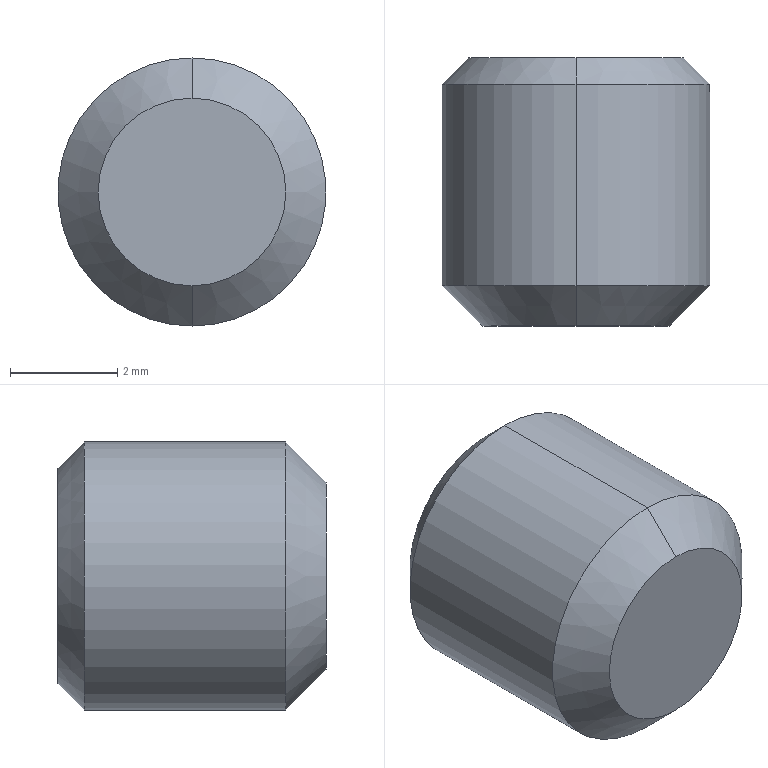Part | STEP file | 0232_Z_HOKW63_3 | 1 solid | 22 faces | box 5 x 5 x 5 mm | volume 80.427 mm3 | plane 14 | cone 6 | cylinder 2 | commonest cylinder face diameters 5 x2
STEP:
#1=CARTESIAN_POINT('',(0.,0.,0.));
#2=DIRECTION('',(0.,0.,1.));
#3=DIRECTION('',(1.,0.,0.));
#4=AXIS2_PLACEMENT_3D('',#1,#2,#3);
#5=CARTESIAN_POINT('',(-9.,17.009,-2.5));
#6=VERTEX_POINT('',#5);
#7=CARTESIAN_POINT('',(-9.,17.009,2.5));
#8=VERTEX_POINT('',#7);
#9=CARTESIAN_POINT('',(-9.,17.009,0.));
#10=DIRECTION('',(0.,-1.,0.));
#11=DIRECTION('',(0.,0.,-1.));
#12=AXIS2_PLACEMENT_3D('',#9,#10,#11);
#13=CIRCLE('',#12,2.5);
#14=CARTESIAN_POINT('',(-9.,15.13,0.));
#15=DIRECTION('',(0.,-1.,0.));
#16=DIRECTION('',(0.,0.,-1.));
#17=AXIS2_PLACEMENT_3D('',#14,#15,#16);
#18=CYLINDRICAL_SURFACE('',#17,2.5);
#19=CARTESIAN_POINT('',(0.,-1.88));
#20=DIRECTION('',(1.,0.));
#21=VECTOR('',#20,1.);
#22=LINE('',#19,#21);
#23=(GEOMETRIC_REPRESENTATION_CONTEXT(2)PARAMETRIC_REPRESENTATION_CONTEXT()REPRESENTATION_CONTEXT('',''));
#24=DEFINITIONAL_REPRESENTATION('',(#22),#23);
#25=PCURVE('',#18,#24);
#26=CARTESIAN_POINT('',(-9.,17.01,0.));
#27=DIRECTION('',(0.,-1.,0.));
#28=DIRECTION('',(0.,0.,-1.));
#29=AXIS2_PLACEMENT_3D('',#26,#27,#28);
#30=CONICAL_SURFACE('',#29,2.5,0.7854);
#31=CARTESIAN_POINT('',(0.,0.));
#32=DIRECTION('',(1.,0.));
#33=VECTOR('',#32,1.);
#34=LINE('',#31,#33);
#35=(GEOMETRIC_REPRESENTATION_CONTEXT(2)PARAMETRIC_REPRESENTATION_CONTEXT()REPRESENTATION_CONTEXT('',''));
#36=DEFINITIONAL_REPRESENTATION('',(#34),#35);
#37=PCURVE('',#30,#36);
#38=SURFACE_CURVE('',#13,(#25,#37),.PCURVE_S1.);
#39=EDGE_CURVE('',#6,#8,#38,.T.);
#40=ORIENTED_EDGE('',*,*,#39,.T.);
#41=CARTESIAN_POINT('',(-9.,13.25,2.5));
#42=VERTEX_POINT('',#41);
#43=CARTESIAN_POINT('',(-9.,15.13,2.5));
#44=DIRECTION('',(0.,-1.,0.));
#45=VECTOR('',#44,1.);
#46=LINE('',#43,#45);
#47=CARTESIAN_POINT('',(3.142,0.));
#48=DIRECTION('',(0.,1.));
#49=VECTOR('',#48,1.);
#50=LINE('',#47,#49);
#51=(GEOMETRIC_REPRESENTATION_CONTEXT(2)PARAMETRIC_REPRESENTATION_CONTEXT()REPRESENTATION_CONTEXT('',''));
#52=DEFINITIONAL_REPRESENTATION('',(#50),#51);
#53=PCURVE('',#18,#52);
#54=CARTESIAN_POINT('',(-9.,15.13,0.));
#55=DIRECTION('',(0.,-1.,0.));
#56=DIRECTION('',(0.,0.,-1.));
#57=AXIS2_PLACEMENT_3D('',#54,#55,#56);
#58=CYLINDRICAL_SURFACE('',#57,2.5);
#59=CARTESIAN_POINT('',(3.142,0.));
#60=DIRECTION('',(0.,1.));
#61=VECTOR('',#60,1.);
#62=LINE('',#59,#61);
#63=(GEOMETRIC_REPRESENTATION_CONTEXT(2)PARAMETRIC_REPRESENTATION_CONTEXT()REPRESENTATION_CONTEXT('',''));
#64=DEFINITIONAL_REPRESENTATION('',(#62),#63);
#65=PCURVE('',#58,#64);
#66=SURFACE_CURVE('',#46,(#53,#65),.PCURVE_S1.);
#67=EDGE_CURVE('',#8,#42,#66,.T.);
#68=ORIENTED_EDGE('',*,*,#67,.T.);
#69=CARTESIAN_POINT('',(-9.,13.25,-2.5));
#70=VERTEX_POINT('',#69);
#71=CARTESIAN_POINT('',(-9.,13.25,0.));
#72=DIRECTION('',(0.,1.,0.));
#73=DIRECTION('',(0.,0.,-1.));
#74=AXIS2_PLACEMENT_3D('',#71,#72,#73);
#75=CIRCLE('',#74,2.5);
#76=CARTESIAN_POINT('',(6.283,1.88));
#77=DIRECTION('',(-1.,0.));
#78=VECTOR('',#77,1.);
#79=LINE('',#76,#78);
#80=(GEOMETRIC_REPRESENTATION_CONTEXT(2)PARAMETRIC_REPRESENTATION_CONTEXT()REPRESENTATION_CONTEXT('',''));
#81=DEFINITIONAL_REPRESENTATION('',(#79),#80);
#82=PCURVE('',#18,#81);
#83=CARTESIAN_POINT('',(-9.,13.25,0.));
#84=DIRECTION('',(0.,1.,0.));
#85=DIRECTION('',(0.,0.,1.));
#86=AXIS2_PLACEMENT_3D('',#83,#84,#85);
#87=CONICAL_SURFACE('',#86,2.5,0.7854);
#88=CARTESIAN_POINT('',(-3.142,0.));
#89=DIRECTION('',(1.,0.));
#90=VECTOR('',#89,1.);
#91=LINE('',#88,#90);
#92=(GEOMETRIC_REPRESENTATION_CONTEXT(2)PARAMETRIC_REPRESENTATION_CONTEXT()REPRESENTATION_CONTEXT('',''));
#93=DEFINITIONAL_REPRESENTATION('',(#91),#92);
#94=PCURVE('',#87,#93);
#95=SURFACE_CURVE('',#75,(#82,#94),.PCURVE_S1.);
#96=EDGE_CURVE('',#42,#70,#95,.T.);
#97=ORIENTED_EDGE('',*,*,#96,.T.);
#98=CARTESIAN_POINT('',(-9.,15.13,-2.5));
#99=DIRECTION('',(0.,-1.,0.));
#100=VECTOR('',#99,1.);
#101=LINE('',#98,#100);
#102=CARTESIAN_POINT('',(0.,0.));
#103=DIRECTION('',(0.,1.));
#104=VECTOR('',#103,1.);
#105=LINE('',#102,#104);
#106=(GEOMETRIC_REPRESENTATION_CONTEXT(2)PARAMETRIC_REPRESENTATION_CONTEXT()REPRESENTATION_CONTEXT('',''));
#107=DEFINITIONAL_REPRESENTATION('',(#105),#106);
#108=PCURVE('',#18,#107);
#109=CARTESIAN_POINT('',(6.283,0.));
#110=DIRECTION('',(0.,1.));
#111=VECTOR('',#110,1.);
#112=LINE('',#109,#111);
#113=(GEOMETRIC_REPRESENTATION_CONTEXT(2)PARAMETRIC_REPRESENTATION_CONTEXT()REPRESENTATION_CONTEXT('',''));
#114=DEFINITIONAL_REPRESENTATION('',(#112),#113);
#115=PCURVE('',#58,#114);
#116=SURFACE_CURVE('',#101,(#108,#115),.PCURVE_S1.);
#117=EDGE_CURVE('',#6,#70,#116,.T.);
#118=ORIENTED_EDGE('',*,*,#117,.F.);
#119=EDGE_LOOP('',(#40,#68,#97,#118));
#120=FACE_BOUND('',#119,.T.);
#121=ADVANCED_FACE('',(#120),#18,.T.);
#122=CARTESIAN_POINT('',(-9.,17.5,-2.009));
#123=VERTEX_POINT('',#122);
#124=CARTESIAN_POINT('',(-9.,17.5,2.009));
#125=VERTEX_POINT('',#124);
#126=CARTESIAN_POINT('',(-9.,17.5,0.));
#127=DIRECTION('',(0.,-1.,0.));
#128=DIRECTION('',(0.,0.,-1.));
#129=AXIS2_PLACEMENT_3D('',#126,#127,#128);
#130=CIRCLE('',#129,2.009);
#131=CARTESIAN_POINT('',(0.,-0.4905));
#132=DIRECTION('',(1.,0.));
#133=VECTOR('',#132,1.);
#134=LINE('',#131,#133);
#135=(GEOMETRIC_REPRESENTATION_CONTEXT(2)PARAMETRIC_REPRESENTATION_CONTEXT()REPRESENTATION_CONTEXT('',''));
#136=DEFINITIONAL_REPRESENTATION('',(#134),#135);
#137=PCURVE('',#30,#136);
#138=CARTESIAN_POINT('',(-9.,17.5,1.005));
#139=DIRECTION('',(0.,1.,0.));
#140=DIRECTION('',(0.,0.,1.));
#141=AXIS2_PLACEMENT_3D('',#138,#139,#140);
#142=PLANE('',#141);
#143=CARTESIAN_POINT('',(-3.014,0.));
#144=CARTESIAN_POINT('',(-3.014,3.481));
#145=CARTESIAN_POINT('',(0.,1.74));
#146=CARTESIAN_POINT('',(3.014,0.));
#147=CARTESIAN_POINT('',(0.,-1.74));
#148=CARTESIAN_POINT('',(-3.014,-3.481));
#149=CARTESIAN_POINT('',(-3.014,0.));
#150=(BOUNDED_CURVE()B_SPLINE_CURVE(2,(#143,#144,#145,#146,#147,#148,#149),.UNSPECIFIED.,.T.,.F.)B_SPLINE_CURVE_WITH_KNOTS((1,2,2,2,2,1),(-2.094,0.,2.094,4.189,6.283,8.378),.UNSPECIFIED.)CURVE()GEOMETRIC_REPRESENTATION_ITEM()RATIONAL_B_SPLINE_CURVE((1.,0.5,1.,0.5,1.,0.5,1.))REPRESENTATION_ITEM(''));
#151=(GEOMETRIC_REPRESENTATION_CONTEXT(2)PARAMETRIC_REPRESENTATION_CONTEXT()REPRESENTATION_CONTEXT('',''));
#152=DEFINITIONAL_REPRESENTATION('',(#150),#151);
#153=PCURVE('',#142,#152);
#154=SURFACE_CURVE('',#130,(#137,#153),.PCURVE_S1.);
#155=EDGE_CURVE('',#123,#125,#154,.T.);
#156=ORIENTED_EDGE('',*,*,#155,.T.);
#157=CARTESIAN_POINT('',(-9.,17.01,2.5));
#158=DIRECTION('',(0.,-0.7071,0.7071));
#159=VECTOR('',#158,1.);
#160=LINE('',#157,#159);
#161=CARTESIAN_POINT('',(3.142,0.));
#162=DIRECTION('',(0.,1.));
#163=VECTOR('',#162,1.);
#164=LINE('',#161,#163);
#165=(GEOMETRIC_REPRESENTATION_CONTEXT(2)PARAMETRIC_REPRESENTATION_CONTEXT()REPRESENTATION_CONTEXT('',''));
#166=DEFINITIONAL_REPRESENTATION('',(#164),#165);
#167=PCURVE('',#30,#166);
#168=CARTESIAN_POINT('',(-9.,17.01,0.));
#169=DIRECTION('',(0.,-1.,0.));
#170=DIRECTION('',(0.,0.,-1.));
#171=AXIS2_PLACEMENT_3D('',#168,#169,#170);
#172=CONICAL_SURFACE('',#171,2.5,0.7854);
#173=CARTESIAN_POINT('',(3.142,0.));
#174=DIRECTION('',(0.,1.));
#175=VECTOR('',#174,1.);
#176=LINE('',#173,#175);
#177=(GEOMETRIC_REPRESENTATION_CONTEXT(2)PARAMETRIC_REPRESENTATION_CONTEXT()REPRESENTATION_CONTEXT('',''));
#178=DEFINITIONAL_REPRESENTATION('',(#176),#177);
#179=PCURVE('',#172,#178);
#180=SURFACE_CURVE('',#160,(#167,#179),.PCURVE_S1.);
#181=EDGE_CURVE('',#125,#8,#180,.T.);
#182=ORIENTED_EDGE('',*,*,#181,.T.);
#183=ORIENTED_EDGE('',*,*,#39,.F.);
#184=CARTESIAN_POINT('',(-9.,17.01,-2.5));
#185=DIRECTION('',(0.,-0.7071,-0.7071));
#186=VECTOR('',#185,1.);
#187=LINE('',#184,#186);
#188=CARTESIAN_POINT('',(0.,0.));
#189=DIRECTION('',(0.,1.));
#190=VECTOR('',#189,1.);
#191=LINE('',#188,#190);
#192=(GEOMETRIC_REPRESENTATION_CONTEXT(2)PARAMETRIC_REPRESENTATION_CONTEXT()REPRESENTATION_CONTEXT('',''));
#193=DEFINITIONAL_REPRESENTATION('',(#191),#192);
#194=PCURVE('',#30,#193);
#195=CARTESIAN_POINT('',(6.283,0.));
#196=DIRECTION('',(0.,1.));
#197=VECTOR('',#196,1.);
#198=LINE('',#195,#197);
#199=(GEOMETRIC_REPRESENTATION_CONTEXT(2)PARAMETRIC_REPRESENTATION_CONTEXT()REPRESENTATION_CONTEXT('',''));
#200=DEFINITIONAL_REPRESENTATION('',(#198),#199);
#201=PCURVE('',#172,#200);
#202=SURFACE_CURVE('',#187,(#194,#201),.PCURVE_S1.);
#203=EDGE_CURVE('',#123,#6,#202,.T.);
#204=ORIENTED_EDGE('',*,*,#203,.F.);
#205=EDGE_LOOP('',(#156,#182,#183,#204));
#206=FACE_BOUND('',#205,.T.);
#207=ADVANCED_FACE('',(#206),#30,.T.);
#208=CARTESIAN_POINT('',(-9.,12.5,1.75));
#209=VERTEX_POINT('',#208);
#210=CARTESIAN_POINT('',(-9.,12.5,-1.75));
#211=VERTEX_POINT('',#210);
#212=CARTESIAN_POINT('',(-9.,12.5,0.));
#213=DIRECTION('',(0.,1.,0.));
#214=DIRECTION('',(0.,0.,1.));
#215=AXIS2_PLACEMENT_3D('',#212,#213,#214);
#216=CIRCLE('',#215,1.75);
#217=CARTESIAN_POINT('',(0.,-0.75));
#218=DIRECTION('',(1.,0.));
#219=VECTOR('',#218,1.);
#220=LINE('',#217,#219);
#221=(GEOMETRIC_REPRESENTATION_CONTEXT(2)PARAMETRIC_REPRESENTATION_CONTEXT()REPRESENTATION_CONTEXT('',''));
#222=DEFINITIONAL_REPRESENTATION('',(#220),#221);
#223=PCURVE('',#87,#222);
#224=CARTESIAN_POINT('',(-9.,12.5,0.875));
#225=DIRECTION('',(0.,-1.,0.));
#226=DIRECTION('',(0.,0.,-1.));
#227=AXIS2_PLACEMENT_3D('',#224,#225,#226);
#228=PLANE('',#227);
#229=CARTESIAN_POINT('',(-0.875,0.));
#230=CARTESIAN_POINT('',(-0.875,3.031));
#231=CARTESIAN_POINT('',(1.75,1.516));
#232=CARTESIAN_POINT('',(4.375,0.));
#233=CARTESIAN_POINT('',(1.75,-1.516));
#234=CARTESIAN_POINT('',(-0.875,-3.031));
#235=CARTESIAN_POINT('',(-0.875,0.));
#236=(BOUNDED_CURVE()B_SPLINE_CURVE(2,(#229,#230,#231,#232,#233,#234,#235),.UNSPECIFIED.,.T.,.F.)B_SPLINE_CURVE_WITH_KNOTS((1,2,2,2,2,1),(-2.094,0.,2.094,4.189,6.283,8.378),.UNSPECIFIED.)CURVE()GEOMETRIC_REPRESENTATION_ITEM()RATIONAL_B_SPLINE_CURVE((1.,0.5,1.,0.5,1.,0.5,1.))REPRESENTATION_ITEM(''));
#237=(GEOMETRIC_REPRESENTATION_CONTEXT(2)PARAMETRIC_REPRESENTATION_CONTEXT()REPRESENTATION_CONTEXT('',''));
#238=DEFINITIONAL_REPRESENTATION('',(#236),#237);
#239=PCURVE('',#228,#238);
#240=SURFACE_CURVE('',#216,(#223,#239),.PCURVE_S1.);
#241=EDGE_CURVE('',#209,#211,#240,.T.);
#242=ORIENTED_EDGE('',*,*,#241,.T.);
#243=CARTESIAN_POINT('',(-9.,13.25,-2.5));
#244=DIRECTION('',(0.,0.7071,-0.7071));
#245=VECTOR('',#244,1.);
#246=LINE('',#243,#245);
#247=CARTESIAN_POINT('',(3.142,0.));
#248=DIRECTION('',(0.,1.));
#249=VECTOR('',#248,1.);
#250=LINE('',#247,#249);
#251=(GEOMETRIC_REPRESENTATION_CONTEXT(2)PARAMETRIC_REPRESENTATION_CONTEXT()REPRESENTATION_CONTEXT('',''));
#252=DEFINITIONAL_REPRESENTATION('',(#250),#251);
#253=PCURVE('',#87,#252);
#254=CARTESIAN_POINT('',(-9.,13.25,0.));
#255=DIRECTION('',(0.,1.,0.));
#256=DIRECTION('',(0.,0.,1.));
#257=AXIS2_PLACEMENT_3D('',#254,#255,#256);
#258=CONICAL_SURFACE('',#257,2.5,0.7854);
#259=CARTESIAN_POINT('',(3.142,0.));
#260=DIRECTION('',(0.,1.));
#261=VECTOR('',#260,1.);
#262=LINE('',#259,#261);
#263=(GEOMETRIC_REPRESENTATION_CONTEXT(2)PARAMETRIC_REPRESENTATION_CONTEXT()REPRESENTATION_CONTEXT('',''));
#264=DEFINITIONAL_REPRESENTATION('',(#262),#263);
#265=PCURVE('',#258,#264);
#266=SURFACE_CURVE('',#246,(#253,#265),.PCURVE_S1.);
#267=EDGE_CURVE('',#211,#70,#266,.T.);
#268=ORIENTED_EDGE('',*,*,#267,.T.);
#269=ORIENTED_EDGE('',*,*,#96,.F.);
#270=CARTESIAN_POINT('',(-9.,13.25,2.5));
#271=DIRECTION('',(0.,0.7071,0.7071));
#272=VECTOR('',#271,1.);
#273=LINE('',#270,#272);
#274=CARTESIAN_POINT('',(0.,0.));
#275=DIRECTION('',(0.,1.));
#276=VECTOR('',#275,1.);
#277=LINE('',#274,#276);
#278=(GEOMETRIC_REPRESENTATION_CONTEXT(2)PARAMETRIC_REPRESENTATION_CONTEXT()REPRESENTATION_CONTEXT('',''));
#279=DEFINITIONAL_REPRESENTATION('',(#277),#278);
#280=PCURVE('',#87,#279);
#281=CARTESIAN_POINT('',(6.283,0.));
#282=DIRECTION('',(0.,1.));
#283=VECTOR('',#282,1.);
#284=LINE('',#281,#283);
#285=(GEOMETRIC_REPRESENTATION_CONTEXT(2)PARAMETRIC_REPRESENTATION_CONTEXT()REPRESENTATION_CONTEXT('',''));
#286=DEFINITIONAL_REPRESENTATION('',(#284),#285);
#287=PCURVE('',#258,#286);
#288=SURFACE_CURVE('',#273,(#280,#287),.PCURVE_S1.);
#289=EDGE_CURVE('',#209,#42,#288,.T.);
#290=ORIENTED_EDGE('',*,*,#289,.F.);
#291=EDGE_LOOP('',(#242,#268,#269,#290));
#292=FACE_BOUND('',#291,.T.);
#293=ADVANCED_FACE('',(#292),#87,.T.);
#294=CARTESIAN_POINT('',(-9.,15.5,1.25));
#295=VERTEX_POINT('',#294);
#296=CARTESIAN_POINT('',(-9.625,15.5,1.083));
#297=VERTEX_POINT('',#296);
#298=CARTESIAN_POINT('',(-9.,15.5,0.));
#299=DIRECTION('',(0.,-1.,0.));
#300=DIRECTION('',(0.,0.,1.));
#301=AXIS2_PLACEMENT_3D('',#298,#299,#300);
#302=CIRCLE('',#301,1.25);
#303=CARTESIAN_POINT('',(-9.,15.5,0.));
#304=DIRECTION('',(0.,1.,0.));
#305=DIRECTION('',(0.,0.,1.));
#306=AXIS2_PLACEMENT_3D('',#303,#304,#305);
#307=CONICAL_SURFACE('',#306,1.25,1.047);
#308=CARTESIAN_POINT('',(6.283,0.));
#309=DIRECTION('',(-1.,0.));
#310=VECTOR('',#309,1.);
#311=LINE('',#308,#310);
#312=(GEOMETRIC_REPRESENTATION_CONTEXT(2)PARAMETRIC_REPRESENTATION_CONTEXT()REPRESENTATION_CONTEXT('',''));
#313=DEFINITIONAL_REPRESENTATION('',(#311),#312);
#314=PCURVE('',#307,#313);
#315=CARTESIAN_POINT('',(-9.,15.5,0.));
#316=DIRECTION('',(0.,-1.,0.));
#317=DIRECTION('',(0.,0.,-1.));
#318=AXIS2_PLACEMENT_3D('',#315,#316,#317);
#319=PLANE('',#318);
#320=CARTESIAN_POINT('',(0.,0.));
#321=DIRECTION('',(-1.,0.));
#322=AXIS2_PLACEMENT_2D('',#320,#321);
#323=CIRCLE('',#322,1.25);
#324=(GEOMETRIC_REPRESENTATION_CONTEXT(2)PARAMETRIC_REPRESENTATION_CONTEXT()REPRESENTATION_CONTEXT('',''));
#325=DEFINITIONAL_REPRESENTATION('',(#323),#324);
#326=PCURVE('',#319,#325);
#327=SURFACE_CURVE('',#302,(#314,#326),.PCURVE_S1.);
#328=EDGE_CURVE('',#295,#297,#327,.T.);
#329=ORIENTED_EDGE('',*,*,#328,.T.);
#330=CARTESIAN_POINT('',(-10.25,15.5,0.));
#331=VERTEX_POINT('',#330);
#332=CARTESIAN_POINT('',(-9.,15.5,0.));
#333=DIRECTION('',(0.,1.,0.));
#334=DIRECTION('',(0.,0.,1.));
#335=AXIS2_PLACEMENT_3D('',#332,#333,#334);
#336=CIRCLE('',#335,1.25);
#337=CARTESIAN_POINT('',(0.,0.));
#338=DIRECTION('',(1.,0.));
#339=VECTOR('',#338,1.);
#340=LINE('',#337,#339);
#341=(GEOMETRIC_REPRESENTATION_CONTEXT(2)PARAMETRIC_REPRESENTATION_CONTEXT()REPRESENTATION_CONTEXT('',''));
#342=DEFINITIONAL_REPRESENTATION('',(#340),#341);
#343=PCURVE('',#307,#342);
#344=CARTESIAN_POINT('',(-9.,15.5,0.));
#345=DIRECTION('',(0.,-1.,0.));
#346=DIRECTION('',(0.,0.,-1.));
#347=AXIS2_PLACEMENT_3D('',#344,#345,#346);
#348=PLANE('',#347);
#349=CARTESIAN_POINT('',(-1.25,0.));
#350=CARTESIAN_POINT('',(-1.25,2.165));
#351=CARTESIAN_POINT('',(0.625,1.083));
#352=CARTESIAN_POINT('',(2.5,0.));
#353=CARTESIAN_POINT('',(0.625,-1.083));
#354=CARTESIAN_POINT('',(-1.25,-2.165));
#355=CARTESIAN_POINT('',(-1.25,0.));
#356=(BOUNDED_CURVE()B_SPLINE_CURVE(2,(#349,#350,#351,#352,#353,#354,#355),.UNSPECIFIED.,.T.,.F.)B_SPLINE_CURVE_WITH_KNOTS((1,2,2,2,2,1),(-2.094,0.,2.094,4.189,6.283,8.378),.UNSPECIFIED.)CURVE()GEOMETRIC_REPRESENTATION_ITEM()RATIONAL_B_SPLINE_CURVE((1.,0.5,1.,0.5,1.,0.5,1.))REPRESENTATION_ITEM(''));
#357=(GEOMETRIC_REPRESENTATION_CONTEXT(2)PARAMETRIC_REPRESENTATION_CONTEXT()REPRESENTATION_CONTEXT('',''));
#358=DEFINITIONAL_REPRESENTATION('',(#356),#357);
#359=PCURVE('',#348,#358);
#360=SURFACE_CURVE('',#336,(#343,#359),.PCURVE_S1.);
#361=EDGE_CURVE('',#331,#297,#360,.T.);
#362=ORIENTED_EDGE('',*,*,#361,.F.);
#363=CARTESIAN_POINT('',(-9.625,15.5,-1.083));
#364=VERTEX_POINT('',#363);
#365=CARTESIAN_POINT('',(-9.,15.5,0.));
#366=DIRECTION('',(0.,-1.,0.));
#367=DIRECTION('',(0.,0.,1.));
#368=AXIS2_PLACEMENT_3D('',#365,#366,#367);
#369=CIRCLE('',#368,1.25);
#370=CARTESIAN_POINT('',(6.283,0.));
#371=DIRECTION('',(-1.,0.));
#372=VECTOR('',#371,1.);
#373=LINE('',#370,#372);
#374=(GEOMETRIC_REPRESENTATION_CONTEXT(2)PARAMETRIC_REPRESENTATION_CONTEXT()REPRESENTATION_CONTEXT('',''));
#375=DEFINITIONAL_REPRESENTATION('',(#373),#374);
#376=PCURVE('',#307,#375);
#377=CARTESIAN_POINT('',(-9.,15.5,0.));
#378=DIRECTION('',(0.,-1.,0.));
#379=DIRECTION('',(0.,0.,-1.));
#380=AXIS2_PLACEMENT_3D('',#377,#378,#379);
#381=PLANE('',#380);
#382=CARTESIAN_POINT('',(0.,0.));
#383=DIRECTION('',(-1.,0.));
#384=AXIS2_PLACEMENT_2D('',#382,#383);
#385=CIRCLE('',#384,1.25);
#386=(GEOMETRIC_REPRESENTATION_CONTEXT(2)PARAMETRIC_REPRESENTATION_CONTEXT()REPRESENTATION_CONTEXT('',''));
#387=DEFINITIONAL_REPRESENTATION('',(#385),#386);
#388=PCURVE('',#381,#387);
#389=SURFACE_CURVE('',#369,(#376,#388),.PCURVE_S1.);
#390=EDGE_CURVE('',#331,#364,#389,.T.);
#391=ORIENTED_EDGE('',*,*,#390,.T.);
#392=CARTESIAN_POINT('',(-9.,15.5,-1.25));
#393=VERTEX_POINT('',#392);
#394=CARTESIAN_POINT('',(-9.,15.5,0.));
#395=DIRECTION('',(0.,-1.,0.));
#396=DIRECTION('',(0.,0.,1.));
#397=AXIS2_PLACEMENT_3D('',#394,#395,#396);
#398=CIRCLE('',#397,1.25);
#399=CARTESIAN_POINT('',(6.283,0.));
#400=DIRECTION('',(-1.,0.));
#401=VECTOR('',#400,1.);
#402=LINE('',#399,#401);
#403=(GEOMETRIC_REPRESENTATION_CONTEXT(2)PARAMETRIC_REPRESENTATION_CONTEXT()REPRESENTATION_CONTEXT('',''));
#404=DEFINITIONAL_REPRESENTATION('',(#402),#403);
#405=PCURVE('',#307,#404);
#406=CARTESIAN_POINT('',(-9.,15.5,0.));
#407=DIRECTION('',(0.,-1.,0.));
#408=DIRECTION('',(0.,0.,-1.));
#409=AXIS2_PLACEMENT_3D('',#406,#407,#408);
#410=PLANE('',#409);
#411=CARTESIAN_POINT('',(0.,0.));
#412=DIRECTION('',(-1.,0.));
#413=AXIS2_PLACEMENT_2D('',#411,#412);
#414=CIRCLE('',#413,1.25);
#415=(GEOMETRIC_REPRESENTATION_CONTEXT(2)PARAMETRIC_REPRESENTATION_CONTEXT()REPRESENTATION_CONTEXT('',''));
#416=DEFINITIONAL_REPRESENTATION('',(#414),#415);
#417=PCURVE('',#410,#416);
#418=SURFACE_CURVE('',#398,(#405,#417),.PCURVE_S1.);
#419=EDGE_CURVE('',#364,#393,#418,.T.);
#420=ORIENTED_EDGE('',*,*,#419,.T.);
#421=CARTESIAN_POINT('',(-9.,14.778,0.));
#422=VERTEX_POINT('',#421);
#423=CARTESIAN_POINT('',(-9.,15.5,-1.25));
#424=DIRECTION('',(0.,0.5,-0.866));
#425=VECTOR('',#424,1.);
#426=LINE('',#423,#425);
#427=CARTESIAN_POINT('',(3.142,0.));
#428=DIRECTION('',(0.,1.));
#429=VECTOR('',#428,1.);
#430=LINE('',#427,#429);
#431=(GEOMETRIC_REPRESENTATION_CONTEXT(2)PARAMETRIC_REPRESENTATION_CONTEXT()REPRESENTATION_CONTEXT('',''));
#432=DEFINITIONAL_REPRESENTATION('',(#430),#431);
#433=PCURVE('',#307,#432);
#434=CARTESIAN_POINT('',(-9.,15.5,0.));
#435=DIRECTION('',(0.,1.,0.));
#436=DIRECTION('',(0.,0.,1.));
#437=AXIS2_PLACEMENT_3D('',#434,#435,#436);
#438=CONICAL_SURFACE('',#437,1.25,1.047);
#439=CARTESIAN_POINT('',(3.142,0.));
#440=DIRECTION('',(0.,1.));
#441=VECTOR('',#440,1.);
#442=LINE('',#439,#441);
#443=(GEOMETRIC_REPRESENTATION_CONTEXT(2)PARAMETRIC_REPRESENTATION_CONTEXT()REPRESENTATION_CONTEXT('',''));
#444=DEFINITIONAL_REPRESENTATION('',(#442),#443);
#445=PCURVE('',#438,#444);
#446=SURFACE_CURVE('',#426,(#433,#445),.PCURVE_S1.);
#447=EDGE_CURVE('',#422,#393,#446,.T.);
#448=ORIENTED_EDGE('',*,*,#447,.F.);
#449=CARTESIAN_POINT('',(-9.,15.5,1.25));
#450=DIRECTION('',(0.,0.5,0.866));
#451=VECTOR('',#450,1.);
#452=LINE('',#449,#451);
#453=CARTESIAN_POINT('',(6.283,0.));
#454=DIRECTION('',(0.,1.));
#455=VECTOR('',#454,1.);
#456=LINE('',#453,#455);
#457=(GEOMETRIC_REPRESENTATION_CONTEXT(2)PARAMETRIC_REPRESENTATION_CONTEXT()REPRESENTATION_CONTEXT('',''));
#458=DEFINITIONAL_REPRESENTATION('',(#456),#457);
#459=PCURVE('',#307,#458);
#460=CARTESIAN_POINT('',(0.,0.));
#461=DIRECTION('',(0.,1.));
#462=VECTOR('',#461,1.);
#463=LINE('',#460,#462);
#464=(GEOMETRIC_REPRESENTATION_CONTEXT(2)PARAMETRIC_REPRESENTATION_CONTEXT()REPRESENTATION_CONTEXT('',''));
#465=DEFINITIONAL_REPRESENTATION('',(#463),#464);
#466=PCURVE('',#438,#465);
#467=SURFACE_CURVE('',#452,(#459,#466),.PCURVE_S1.);
#468=EDGE_CURVE('',#422,#295,#467,.T.);
#469=ORIENTED_EDGE('',*,*,#468,.T.);
#470=EDGE_LOOP('',(#329,#362,#391,#420,#448,#469));
#471=FACE_BOUND('',#470,.F.);
#472=ADVANCED_FACE('',(#471),#307,.F.);
#473=ORIENTED_EDGE('',*,*,#67,.F.);
#474=CARTESIAN_POINT('',(-9.,17.009,0.));
#475=DIRECTION('',(0.,-1.,0.));
#476=DIRECTION('',(0.,0.,-1.));
#477=AXIS2_PLACEMENT_3D('',#474,#475,#476);
#478=CIRCLE('',#477,2.5);
#479=CARTESIAN_POINT('',(0.,-1.88));
#480=DIRECTION('',(1.,0.));
#481=VECTOR('',#480,1.);
#482=LINE('',#479,#481);
#483=(GEOMETRIC_REPRESENTATION_CONTEXT(2)PARAMETRIC_REPRESENTATION_CONTEXT()REPRESENTATION_CONTEXT('',''));
#484=DEFINITIONAL_REPRESENTATION('',(#482),#483);
#485=PCURVE('',#58,#484);
#486=CARTESIAN_POINT('',(0.,0.));
#487=DIRECTION('',(1.,0.));
#488=VECTOR('',#487,1.);
#489=LINE('',#486,#488);
#490=(GEOMETRIC_REPRESENTATION_CONTEXT(2)PARAMETRIC_REPRESENTATION_CONTEXT()REPRESENTATION_CONTEXT('',''));
#491=DEFINITIONAL_REPRESENTATION('',(#489),#490);
#492=PCURVE('',#172,#491);
#493=SURFACE_CURVE('',#478,(#485,#492),.PCURVE_S1.);
#494=EDGE_CURVE('',#8,#6,#493,.T.);
#495=ORIENTED_EDGE('',*,*,#494,.T.);
#496=ORIENTED_EDGE('',*,*,#117,.T.);
#497=CARTESIAN_POINT('',(-9.,13.25,0.));
#498=DIRECTION('',(0.,1.,0.));
#499=DIRECTION('',(0.,0.,-1.));
#500=AXIS2_PLACEMENT_3D('',#497,#498,#499);
#501=CIRCLE('',#500,2.5);
#502=CARTESIAN_POINT('',(6.283,1.88));
#503=DIRECTION('',(-1.,0.));
#504=VECTOR('',#503,1.);
#505=LINE('',#502,#504);
#506=(GEOMETRIC_REPRESENTATION_CONTEXT(2)PARAMETRIC_REPRESENTATION_CONTEXT()REPRESENTATION_CONTEXT('',''));
#507=DEFINITIONAL_REPRESENTATION('',(#505),#506);
#508=PCURVE('',#58,#507);
#509=CARTESIAN_POINT('',(3.142,0.));
#510=DIRECTION('',(1.,0.));
#511=VECTOR('',#510,1.);
#512=LINE('',#509,#511);
#513=(GEOMETRIC_REPRESENTATION_CONTEXT(2)PARAMETRIC_REPRESENTATION_CONTEXT()REPRESENTATION_CONTEXT('',''));
#514=DEFINITIONAL_REPRESENTATION('',(#512),#513);
#515=PCURVE('',#258,#514);
#516=SURFACE_CURVE('',#501,(#508,#515),.PCURVE_S1.);
#517=EDGE_CURVE('',#70,#42,#516,.T.);
#518=ORIENTED_EDGE('',*,*,#517,.T.);
#519=EDGE_LOOP('',(#473,#495,#496,#518));
#520=FACE_BOUND('',#519,.T.);
#521=ADVANCED_FACE('',(#520),#58,.T.);
#522=ORIENTED_EDGE('',*,*,#181,.F.);
#523=CARTESIAN_POINT('',(-9.,17.5,0.));
#524=DIRECTION('',(0.,-1.,0.));
#525=DIRECTION('',(0.,0.,-1.));
#526=AXIS2_PLACEMENT_3D('',#523,#524,#525);
#527=CIRCLE('',#526,2.009);
#528=CARTESIAN_POINT('',(0.,-0.4905));
#529=DIRECTION('',(1.,0.));
#530=VECTOR('',#529,1.);
#531=LINE('',#528,#530);
#532=(GEOMETRIC_REPRESENTATION_CONTEXT(2)PARAMETRIC_REPRESENTATION_CONTEXT()REPRESENTATION_CONTEXT('',''));
#533=DEFINITIONAL_REPRESENTATION('',(#531),#532);
#534=PCURVE('',#172,#533);
#535=CARTESIAN_POINT('',(-3.014,0.));
#536=CARTESIAN_POINT('',(-3.014,3.481));
#537=CARTESIAN_POINT('',(0.,1.74));
#538=CARTESIAN_POINT('',(3.014,0.));
#539=CARTESIAN_POINT('',(0.,-1.74));
#540=CARTESIAN_POINT('',(-3.014,-3.481));
#541=CARTESIAN_POINT('',(-3.014,0.));
#542=(BOUNDED_CURVE()B_SPLINE_CURVE(2,(#535,#536,#537,#538,#539,#540,#541),.UNSPECIFIED.,.T.,.F.)B_SPLINE_CURVE_WITH_KNOTS((1,2,2,2,2,1),(-2.094,0.,2.094,4.189,6.283,8.378),.UNSPECIFIED.)CURVE()GEOMETRIC_REPRESENTATION_ITEM()RATIONAL_B_SPLINE_CURVE((1.,0.5,1.,0.5,1.,0.5,1.))REPRESENTATION_ITEM(''));
#543=(GEOMETRIC_REPRESENTATION_CONTEXT(2)PARAMETRIC_REPRESENTATION_CONTEXT()REPRESENTATION_CONTEXT('',''));
#544=DEFINITIONAL_REPRESENTATION('',(#542),#543);
#545=PCURVE('',#142,#544);
#546=SURFACE_CURVE('',#527,(#534,#545),.PCURVE_S1.);
#547=EDGE_CURVE('',#125,#123,#546,.T.);
#548=ORIENTED_EDGE('',*,*,#547,.T.);
#549=ORIENTED_EDGE('',*,*,#203,.T.);
#550=ORIENTED_EDGE('',*,*,#494,.F.);
#551=EDGE_LOOP('',(#522,#548,#549,#550));
#552=FACE_BOUND('',#551,.T.);
#553=ADVANCED_FACE('',(#552),#172,.T.);
#554=ORIENTED_EDGE('',*,*,#267,.F.);
#555=CARTESIAN_POINT('',(-9.,12.5,0.));
#556=DIRECTION('',(0.,1.,0.));
#557=DIRECTION('',(0.,0.,1.));
#558=AXIS2_PLACEMENT_3D('',#555,#556,#557);
#559=CIRCLE('',#558,1.75);
#560=CARTESIAN_POINT('',(0.,-0.75));
#561=DIRECTION('',(1.,0.));
#562=VECTOR('',#561,1.);
#563=LINE('',#560,#562);
#564=(GEOMETRIC_REPRESENTATION_CONTEXT(2)PARAMETRIC_REPRESENTATION_CONTEXT()REPRESENTATION_CONTEXT('',''));
#565=DEFINITIONAL_REPRESENTATION('',(#563),#564);
#566=PCURVE('',#258,#565);
#567=CARTESIAN_POINT('',(-0.875,0.));
#568=CARTESIAN_POINT('',(-0.875,3.031));
#569=CARTESIAN_POINT('',(1.75,1.516));
#570=CARTESIAN_POINT('',(4.375,0.));
#571=CARTESIAN_POINT('',(1.75,-1.516));
#572=CARTESIAN_POINT('',(-0.875,-3.031));
#573=CARTESIAN_POINT('',(-0.875,0.));
#574=(BOUNDED_CURVE()B_SPLINE_CURVE(2,(#567,#568,#569,#570,#571,#572,#573),.UNSPECIFIED.,.T.,.F.)B_SPLINE_CURVE_WITH_KNOTS((1,2,2,2,2,1),(-2.094,0.,2.094,4.189,6.283,8.378),.UNSPECIFIED.)CURVE()GEOMETRIC_REPRESENTATION_ITEM()RATIONAL_B_SPLINE_CURVE((1.,0.5,1.,0.5,1.,0.5,1.))REPRESENTATION_ITEM(''));
#575=(GEOMETRIC_REPRESENTATION_CONTEXT(2)PARAMETRIC_REPRESENTATION_CONTEXT()REPRESENTATION_CONTEXT('',''));
#576=DEFINITIONAL_REPRESENTATION('',(#574),#575);
#577=PCURVE('',#228,#576);
#578=SURFACE_CURVE('',#559,(#566,#577),.PCURVE_S1.);
#579=EDGE_CURVE('',#211,#209,#578,.T.);
#580=ORIENTED_EDGE('',*,*,#579,.T.);
#581=ORIENTED_EDGE('',*,*,#289,.T.);
#582=ORIENTED_EDGE('',*,*,#517,.F.);
#583=EDGE_LOOP('',(#554,#580,#581,#582));
#584=FACE_BOUND('',#583,.T.);
#585=ADVANCED_FACE('',(#584),#258,.T.);
#586=ORIENTED_EDGE('',*,*,#155,.F.);
#587=ORIENTED_EDGE('',*,*,#547,.F.);
#588=EDGE_LOOP('',(#586,#587));
#589=FACE_BOUND('',#588,.T.);
#590=CARTESIAN_POINT('',(-7.75,17.5,-0.7217));
#591=VERTEX_POINT('',#590);
#592=CARTESIAN_POINT('',(-7.75,17.5,0.7217));
#593=VERTEX_POINT('',#592);
#594=CARTESIAN_POINT('',(-7.75,17.5,0.7217));
#595=DIRECTION('',(0.,0.,1.));
#596=VECTOR('',#595,1.);
#597=LINE('',#594,#596);
#598=CARTESIAN_POINT('',(-0.2831,1.25));
#599=DIRECTION('',(1.,0.));
#600=VECTOR('',#599,1.);
#601=LINE('',#598,#600);
#602=(GEOMETRIC_REPRESENTATION_CONTEXT(2)PARAMETRIC_REPRESENTATION_CONTEXT()REPRESENTATION_CONTEXT('',''));
#603=DEFINITIONAL_REPRESENTATION('',(#601),#602);
#604=PCURVE('',#142,#603);
#605=CARTESIAN_POINT('',(-7.75,17.5,0.7217));
#606=DIRECTION('',(1.,0.,0.));
#607=DIRECTION('',(0.,0.,-1.));
#608=AXIS2_PLACEMENT_3D('',#605,#606,#607);
#609=PLANE('',#608);
#610=CARTESIAN_POINT('',(0.,0.));
#611=DIRECTION('',(-1.,0.));
#612=VECTOR('',#611,1.);
#613=LINE('',#610,#612);
#614=(GEOMETRIC_REPRESENTATION_CONTEXT(2)PARAMETRIC_REPRESENTATION_CONTEXT()REPRESENTATION_CONTEXT('',''));
#615=DEFINITIONAL_REPRESENTATION('',(#613),#614);
#616=PCURVE('',#609,#615);
#617=SURFACE_CURVE('',#597,(#604,#616),.PCURVE_S1.);
#618=EDGE_CURVE('',#591,#593,#617,.T.);
#619=ORIENTED_EDGE('',*,*,#618,.T.);
#620=CARTESIAN_POINT('',(-9.,17.5,1.443));
#621=VERTEX_POINT('',#620);
#622=CARTESIAN_POINT('',(-7.75,17.5,0.7217));
#623=DIRECTION('',(-0.866,0.,0.5));
#624=VECTOR('',#623,1.);
#625=LINE('',#622,#624);
#626=CARTESIAN_POINT('',(-0.2831,1.25));
#627=DIRECTION('',(0.5,-0.866));
#628=VECTOR('',#627,1.);
#629=LINE('',#626,#628);
#630=(GEOMETRIC_REPRESENTATION_CONTEXT(2)PARAMETRIC_REPRESENTATION_CONTEXT()REPRESENTATION_CONTEXT('',''));
#631=DEFINITIONAL_REPRESENTATION('',(#629),#630);
#632=PCURVE('',#142,#631);
#633=CARTESIAN_POINT('',(-9.,17.5,1.443));
#634=DIRECTION('',(0.5,0.,0.866));
#635=DIRECTION('',(0.866,0.,-0.5));
#636=AXIS2_PLACEMENT_3D('',#633,#634,#635);
#637=PLANE('',#636);
#638=CARTESIAN_POINT('',(1.443,0.));
#639=DIRECTION('',(-1.,0.));
#640=VECTOR('',#639,1.);
#641=LINE('',#638,#640);
#642=(GEOMETRIC_REPRESENTATION_CONTEXT(2)PARAMETRIC_REPRESENTATION_CONTEXT()REPRESENTATION_CONTEXT('',''));
#643=DEFINITIONAL_REPRESENTATION('',(#641),#642);
#644=PCURVE('',#637,#643);
#645=SURFACE_CURVE('',#625,(#632,#644),.PCURVE_S1.);
#646=EDGE_CURVE('',#593,#621,#645,.T.);
#647=ORIENTED_EDGE('',*,*,#646,.T.);
#648=CARTESIAN_POINT('',(-10.25,17.5,0.7217));
#649=VERTEX_POINT('',#648);
#650=CARTESIAN_POINT('',(-10.25,17.5,0.7217));
#651=DIRECTION('',(-0.866,0.,-0.5));
#652=VECTOR('',#651,1.);
#653=LINE('',#650,#652);
#654=CARTESIAN_POINT('',(-0.2831,-1.25));
#655=DIRECTION('',(-0.5,-0.866));
#656=VECTOR('',#655,1.);
#657=LINE('',#654,#656);
#658=(GEOMETRIC_REPRESENTATION_CONTEXT(2)PARAMETRIC_REPRESENTATION_CONTEXT()REPRESENTATION_CONTEXT('',''));
#659=DEFINITIONAL_REPRESENTATION('',(#657),#658);
#660=PCURVE('',#142,#659);
#661=CARTESIAN_POINT('',(-10.25,17.5,0.7217));
#662=DIRECTION('',(-0.5,0.,0.866));
#663=DIRECTION('',(0.866,0.,0.5));
#664=AXIS2_PLACEMENT_3D('',#661,#662,#663);
#665=PLANE('',#664);
#666=CARTESIAN_POINT('',(0.,0.));
#667=DIRECTION('',(-1.,0.));
#668=VECTOR('',#667,1.);
#669=LINE('',#666,#668);
#670=(GEOMETRIC_REPRESENTATION_CONTEXT(2)PARAMETRIC_REPRESENTATION_CONTEXT()REPRESENTATION_CONTEXT('',''));
#671=DEFINITIONAL_REPRESENTATION('',(#669),#670);
#672=PCURVE('',#665,#671);
#673=SURFACE_CURVE('',#653,(#660,#672),.PCURVE_S1.);
#674=EDGE_CURVE('',#621,#649,#673,.T.);
#675=ORIENTED_EDGE('',*,*,#674,.T.);
#676=CARTESIAN_POINT('',(-10.25,17.5,-0.7217));
#677=VERTEX_POINT('',#676);
#678=CARTESIAN_POINT('',(-10.25,17.5,-0.7217));
#679=DIRECTION('',(0.,0.,-1.));
#680=VECTOR('',#679,1.);
#681=LINE('',#678,#680);
#682=CARTESIAN_POINT('',(-1.726,-1.25));
#683=DIRECTION('',(-1.,0.));
#684=VECTOR('',#683,1.);
#685=LINE('',#682,#684);
#686=(GEOMETRIC_REPRESENTATION_CONTEXT(2)PARAMETRIC_REPRESENTATION_CONTEXT()REPRESENTATION_CONTEXT('',''));
#687=DEFINITIONAL_REPRESENTATION('',(#685),#686);
#688=PCURVE('',#142,#687);
#689=CARTESIAN_POINT('',(-10.25,17.5,-0.7217));
#690=DIRECTION('',(-1.,0.,0.));
#691=DIRECTION('',(0.,0.,1.));
#692=AXIS2_PLACEMENT_3D('',#689,#690,#691);
#693=PLANE('',#692);
#694=CARTESIAN_POINT('',(0.,0.));
#695=DIRECTION('',(-1.,0.));
#696=VECTOR('',#695,1.);
#697=LINE('',#694,#696);
#698=(GEOMETRIC_REPRESENTATION_CONTEXT(2)PARAMETRIC_REPRESENTATION_CONTEXT()REPRESENTATION_CONTEXT('',''));
#699=DEFINITIONAL_REPRESENTATION('',(#697),#698);
#700=PCURVE('',#693,#699);
#701=SURFACE_CURVE('',#681,(#688,#700),.PCURVE_S1.);
#702=EDGE_CURVE('',#649,#677,#701,.T.);
#703=ORIENTED_EDGE('',*,*,#702,.T.);
#704=CARTESIAN_POINT('',(-9.,17.5,-1.443));
#705=VERTEX_POINT('',#704);
#706=CARTESIAN_POINT('',(-9.,17.5,-1.443));
#707=DIRECTION('',(0.866,0.,-0.5));
#708=VECTOR('',#707,1.);
#709=LINE('',#706,#708);
#710=CARTESIAN_POINT('',(-2.448,0.));
#711=DIRECTION('',(-0.5,0.866));
#712=VECTOR('',#711,1.);
#713=LINE('',#710,#712);
#714=(GEOMETRIC_REPRESENTATION_CONTEXT(2)PARAMETRIC_REPRESENTATION_CONTEXT()REPRESENTATION_CONTEXT('',''));
#715=DEFINITIONAL_REPRESENTATION('',(#713),#714);
#716=PCURVE('',#142,#715);
#717=CARTESIAN_POINT('',(-9.,17.5,-1.443));
#718=DIRECTION('',(-0.5,0.,-0.866));
#719=DIRECTION('',(-0.866,0.,0.5));
#720=AXIS2_PLACEMENT_3D('',#717,#718,#719);
#721=PLANE('',#720);
#722=CARTESIAN_POINT('',(0.,0.));
#723=DIRECTION('',(-1.,0.));
#724=VECTOR('',#723,1.);
#725=LINE('',#722,#724);
#726=(GEOMETRIC_REPRESENTATION_CONTEXT(2)PARAMETRIC_REPRESENTATION_CONTEXT()REPRESENTATION_CONTEXT('',''));
#727=DEFINITIONAL_REPRESENTATION('',(#725),#726);
#728=PCURVE('',#721,#727);
#729=SURFACE_CURVE('',#709,(#716,#728),.PCURVE_S1.);
#730=EDGE_CURVE('',#677,#705,#729,.T.);
#731=ORIENTED_EDGE('',*,*,#730,.T.);
#732=CARTESIAN_POINT('',(-7.75,17.5,-0.7217));
#733=DIRECTION('',(0.866,0.,0.5));
#734=VECTOR('',#733,1.);
#735=LINE('',#732,#734);
#736=CARTESIAN_POINT('',(-1.726,1.25));
#737=DIRECTION('',(0.5,0.866));
#738=VECTOR('',#737,1.);
#739=LINE('',#736,#738);
#740=(GEOMETRIC_REPRESENTATION_CONTEXT(2)PARAMETRIC_REPRESENTATION_CONTEXT()REPRESENTATION_CONTEXT('',''));
#741=DEFINITIONAL_REPRESENTATION('',(#739),#740);
#742=PCURVE('',#142,#741);
#743=CARTESIAN_POINT('',(-7.75,17.5,-0.7217));
#744=DIRECTION('',(0.5,0.,-0.866));
#745=DIRECTION('',(-0.866,0.,-0.5));
#746=AXIS2_PLACEMENT_3D('',#743,#744,#745);
#747=PLANE('',#746);
#748=CARTESIAN_POINT('',(0.,0.));
#749=DIRECTION('',(-1.,0.));
#750=VECTOR('',#749,1.);
#751=LINE('',#748,#750);
#752=(GEOMETRIC_REPRESENTATION_CONTEXT(2)PARAMETRIC_REPRESENTATION_CONTEXT()REPRESENTATION_CONTEXT('',''));
#753=DEFINITIONAL_REPRESENTATION('',(#751),#752);
#754=PCURVE('',#747,#753);
#755=SURFACE_CURVE('',#735,(#742,#754),.PCURVE_S1.);
#756=EDGE_CURVE('',#705,#591,#755,.T.);
#757=ORIENTED_EDGE('',*,*,#756,.T.);
#758=EDGE_LOOP('',(#619,#647,#675,#703,#731,#757));
#759=FACE_BOUND('',#758,.T.);
#760=ADVANCED_FACE('',(#589,#759),#142,.T.);
#761=ORIENTED_EDGE('',*,*,#241,.F.);
#762=ORIENTED_EDGE('',*,*,#579,.F.);
#763=EDGE_LOOP('',(#761,#762));
#764=FACE_BOUND('',#763,.T.);
#765=ADVANCED_FACE('',(#764),#228,.T.);
#766=CARTESIAN_POINT('',(-9.,15.5,1.443));
#767=VERTEX_POINT('',#766);
#768=CARTESIAN_POINT('',(-9.,17.5,1.443));
#769=DIRECTION('',(0.,-1.,0.));
#770=VECTOR('',#769,1.);
#771=LINE('',#768,#770);
#772=CARTESIAN_POINT('',(0.,0.));
#773=DIRECTION('',(0.,-1.));
#774=VECTOR('',#773,1.);
#775=LINE('',#772,#774);
#776=(GEOMETRIC_REPRESENTATION_CONTEXT(2)PARAMETRIC_REPRESENTATION_CONTEXT()REPRESENTATION_CONTEXT('',''));
#777=DEFINITIONAL_REPRESENTATION('',(#775),#776);
#778=PCURVE('',#637,#777);
#779=CARTESIAN_POINT('',(1.443,0.));
#780=DIRECTION('',(0.,-1.));
#781=VECTOR('',#780,1.);
#782=LINE('',#779,#781);
#783=(GEOMETRIC_REPRESENTATION_CONTEXT(2)PARAMETRIC_REPRESENTATION_CONTEXT()REPRESENTATION_CONTEXT('',''));
#784=DEFINITIONAL_REPRESENTATION('',(#782),#783);
#785=PCURVE('',#665,#784);
#786=SURFACE_CURVE('',#771,(#778,#785),.PCURVE_S1.);
#787=EDGE_CURVE('',#621,#767,#786,.T.);
#788=ORIENTED_EDGE('',*,*,#787,.F.);
#789=ORIENTED_EDGE('',*,*,#646,.F.);
#790=CARTESIAN_POINT('',(-7.75,15.5,0.7217));
#791=VERTEX_POINT('',#790);
#792=CARTESIAN_POINT('',(-7.75,17.5,0.7217));
#793=DIRECTION('',(0.,1.,0.));
#794=VECTOR('',#793,1.);
#795=LINE('',#792,#794);
#796=CARTESIAN_POINT('',(1.443,0.));
#797=DIRECTION('',(0.,1.));
#798=VECTOR('',#797,1.);
#799=LINE('',#796,#798);
#800=(GEOMETRIC_REPRESENTATION_CONTEXT(2)PARAMETRIC_REPRESENTATION_CONTEXT()REPRESENTATION_CONTEXT('',''));
#801=DEFINITIONAL_REPRESENTATION('',(#799),#800);
#802=PCURVE('',#637,#801);
#803=CARTESIAN_POINT('',(0.,0.));
#804=DIRECTION('',(0.,1.));
#805=VECTOR('',#804,1.);
#806=LINE('',#803,#805);
#807=(GEOMETRIC_REPRESENTATION_CONTEXT(2)PARAMETRIC_REPRESENTATION_CONTEXT()REPRESENTATION_CONTEXT('',''));
#808=DEFINITIONAL_REPRESENTATION('',(#806),#807);
#809=PCURVE('',#609,#808);
#810=SURFACE_CURVE('',#795,(#802,#809),.PCURVE_S1.);
#811=EDGE_CURVE('',#791,#593,#810,.T.);
#812=ORIENTED_EDGE('',*,*,#811,.F.);
#813=CARTESIAN_POINT('',(-8.375,15.5,1.083));
#814=VERTEX_POINT('',#813);
#815=CARTESIAN_POINT('',(-9.,15.5,1.443));
#816=DIRECTION('',(0.866,0.,-0.5));
#817=VECTOR('',#816,1.);
#818=LINE('',#815,#817);
#819=CARTESIAN_POINT('',(0.,-2.));
#820=DIRECTION('',(1.,0.));
#821=VECTOR('',#820,1.);
#822=LINE('',#819,#821);
#823=(GEOMETRIC_REPRESENTATION_CONTEXT(2)PARAMETRIC_REPRESENTATION_CONTEXT()REPRESENTATION_CONTEXT('',''));
#824=DEFINITIONAL_REPRESENTATION('',(#822),#823);
#825=PCURVE('',#637,#824);
#826=CARTESIAN_POINT('',(-9.,15.5,0.));
#827=DIRECTION('',(0.,-1.,0.));
#828=DIRECTION('',(0.,0.,-1.));
#829=AXIS2_PLACEMENT_3D('',#826,#827,#828);
#830=PLANE('',#829);
#831=CARTESIAN_POINT('',(-1.443,0.));
#832=DIRECTION('',(0.5,0.866));
#833=VECTOR('',#832,1.);
#834=LINE('',#831,#833);
#835=(GEOMETRIC_REPRESENTATION_CONTEXT(2)PARAMETRIC_REPRESENTATION_CONTEXT()REPRESENTATION_CONTEXT('',''));
#836=DEFINITIONAL_REPRESENTATION('',(#834),#835);
#837=PCURVE('',#830,#836);
#838=SURFACE_CURVE('',#818,(#825,#837),.PCURVE_S1.);
#839=EDGE_CURVE('',#814,#791,#838,.T.);
#840=ORIENTED_EDGE('',*,*,#839,.F.);
#841=CARTESIAN_POINT('',(-9.,15.5,1.443));
#842=DIRECTION('',(0.866,0.,-0.5));
#843=VECTOR('',#842,1.);
#844=LINE('',#841,#843);
#845=CARTESIAN_POINT('',(0.,-2.));
#846=DIRECTION('',(1.,0.));
#847=VECTOR('',#846,1.);
#848=LINE('',#845,#847);
#849=(GEOMETRIC_REPRESENTATION_CONTEXT(2)PARAMETRIC_REPRESENTATION_CONTEXT()REPRESENTATION_CONTEXT('',''));
#850=DEFINITIONAL_REPRESENTATION('',(#848),#849);
#851=PCURVE('',#637,#850);
#852=CARTESIAN_POINT('',(-1.443,0.));
#853=DIRECTION('',(0.5,0.866));
#854=VECTOR('',#853,1.);
#855=LINE('',#852,#854);
#856=(GEOMETRIC_REPRESENTATION_CONTEXT(2)PARAMETRIC_REPRESENTATION_CONTEXT()REPRESENTATION_CONTEXT('',''));
#857=DEFINITIONAL_REPRESENTATION('',(#855),#856);
#858=PCURVE('',#319,#857);
#859=SURFACE_CURVE('',#844,(#851,#858),.PCURVE_S1.);
#860=EDGE_CURVE('',#767,#814,#859,.T.);
#861=ORIENTED_EDGE('',*,*,#860,.F.);
#862=EDGE_LOOP('',(#788,#789,#812,#840,#861));
#863=FACE_BOUND('',#862,.T.);
#864=ADVANCED_FACE('',(#863),#637,.F.);
#865=CARTESIAN_POINT('',(-9.,15.5,0.));
#866=DIRECTION('',(0.,-1.,0.));
#867=DIRECTION('',(0.,0.,1.));
#868=AXIS2_PLACEMENT_3D('',#865,#866,#867);
#869=CIRCLE('',#868,1.25);
#870=CARTESIAN_POINT('',(0.,0.));
#871=DIRECTION('',(-1.,0.));
#872=AXIS2_PLACEMENT_2D('',#870,#871);
#873=CIRCLE('',#872,1.25);
#874=(GEOMETRIC_REPRESENTATION_CONTEXT(2)PARAMETRIC_REPRESENTATION_CONTEXT()REPRESENTATION_CONTEXT('',''));
#875=DEFINITIONAL_REPRESENTATION('',(#873),#874);
#876=PCURVE('',#319,#875);
#877=CARTESIAN_POINT('',(6.283,0.));
#878=DIRECTION('',(-1.,0.));
#879=VECTOR('',#878,1.);
#880=LINE('',#877,#879);
#881=(GEOMETRIC_REPRESENTATION_CONTEXT(2)PARAMETRIC_REPRESENTATION_CONTEXT()REPRESENTATION_CONTEXT('',''));
#882=DEFINITIONAL_REPRESENTATION('',(#880),#881);
#883=PCURVE('',#438,#882);
#884=SURFACE_CURVE('',#869,(#876,#883),.PCURVE_S1.);
#885=EDGE_CURVE('',#814,#295,#884,.T.);
#886=ORIENTED_EDGE('',*,*,#885,.T.);
#887=ORIENTED_EDGE('',*,*,#328,.T.);
#888=CARTESIAN_POINT('',(-9.,15.5,1.443));
#889=DIRECTION('',(-0.866,0.,-0.5));
#890=VECTOR('',#889,1.);
#891=LINE('',#888,#890);
#892=CARTESIAN_POINT('',(-1.443,0.));
#893=DIRECTION('',(0.5,-0.866));
#894=VECTOR('',#893,1.);
#895=LINE('',#892,#894);
#896=(GEOMETRIC_REPRESENTATION_CONTEXT(2)PARAMETRIC_REPRESENTATION_CONTEXT()REPRESENTATION_CONTEXT('',''));
#897=DEFINITIONAL_REPRESENTATION('',(#895),#896);
#898=PCURVE('',#319,#897);
#899=CARTESIAN_POINT('',(1.443,-2.));
#900=DIRECTION('',(-1.,0.));
#901=VECTOR('',#900,1.);
#902=LINE('',#899,#901);
#903=(GEOMETRIC_REPRESENTATION_CONTEXT(2)PARAMETRIC_REPRESENTATION_CONTEXT()REPRESENTATION_CONTEXT('',''));
#904=DEFINITIONAL_REPRESENTATION('',(#902),#903);
#905=PCURVE('',#665,#904);
#906=SURFACE_CURVE('',#891,(#898,#905),.PCURVE_S1.);
#907=EDGE_CURVE('',#767,#297,#906,.T.);
#908=ORIENTED_EDGE('',*,*,#907,.F.);
#909=ORIENTED_EDGE('',*,*,#860,.T.);
#910=EDGE_LOOP('',(#886,#887,#908,#909));
#911=FACE_BOUND('',#910,.T.);
#912=ADVANCED_FACE('',(#911),#319,.F.);
#913=CARTESIAN_POINT('',(-10.25,15.5,0.7217));
#914=VERTEX_POINT('',#913);
#915=CARTESIAN_POINT('',(-10.25,17.5,0.7217));
#916=DIRECTION('',(0.,-1.,0.));
#917=VECTOR('',#916,1.);
#918=LINE('',#915,#917);
#919=CARTESIAN_POINT('',(0.,0.));
#920=DIRECTION('',(0.,-1.));
#921=VECTOR('',#920,1.);
#922=LINE('',#919,#921);
#923=(GEOMETRIC_REPRESENTATION_CONTEXT(2)PARAMETRIC_REPRESENTATION_CONTEXT()REPRESENTATION_CONTEXT('',''));
#924=DEFINITIONAL_REPRESENTATION('',(#922),#923);
#925=PCURVE('',#665,#924);
#926=CARTESIAN_POINT('',(1.443,0.));
#927=DIRECTION('',(0.,-1.));
#928=VECTOR('',#927,1.);
#929=LINE('',#926,#928);
#930=(GEOMETRIC_REPRESENTATION_CONTEXT(2)PARAMETRIC_REPRESENTATION_CONTEXT()REPRESENTATION_CONTEXT('',''));
#931=DEFINITIONAL_REPRESENTATION('',(#929),#930);
#932=PCURVE('',#693,#931);
#933=SURFACE_CURVE('',#918,(#925,#932),.PCURVE_S1.);
#934=EDGE_CURVE('',#649,#914,#933,.T.);
#935=ORIENTED_EDGE('',*,*,#934,.F.);
#936=ORIENTED_EDGE('',*,*,#674,.F.);
#937=ORIENTED_EDGE('',*,*,#787,.T.);
#938=ORIENTED_EDGE('',*,*,#907,.T.);
#939=CARTESIAN_POINT('',(-10.25,15.5,0.7217));
#940=DIRECTION('',(0.866,0.,0.5));
#941=VECTOR('',#940,1.);
#942=LINE('',#939,#941);
#943=CARTESIAN_POINT('',(0.,-2.));
#944=DIRECTION('',(1.,0.));
#945=VECTOR('',#944,1.);
#946=LINE('',#943,#945);
#947=(GEOMETRIC_REPRESENTATION_CONTEXT(2)PARAMETRIC_REPRESENTATION_CONTEXT()REPRESENTATION_CONTEXT('',''));
#948=DEFINITIONAL_REPRESENTATION('',(#946),#947);
#949=PCURVE('',#665,#948);
#950=CARTESIAN_POINT('',(-0.7217,-1.25));
#951=DIRECTION('',(-0.5,0.866));
#952=VECTOR('',#951,1.);
#953=LINE('',#950,#952);
#954=(GEOMETRIC_REPRESENTATION_CONTEXT(2)PARAMETRIC_REPRESENTATION_CONTEXT()REPRESENTATION_CONTEXT('',''));
#955=DEFINITIONAL_REPRESENTATION('',(#953),#954);
#956=PCURVE('',#348,#955);
#957=SURFACE_CURVE('',#942,(#949,#956),.PCURVE_S1.);
#958=EDGE_CURVE('',#914,#297,#957,.T.);
#959=ORIENTED_EDGE('',*,*,#958,.F.);
#960=EDGE_LOOP('',(#935,#936,#937,#938,#959));
#961=FACE_BOUND('',#960,.T.);
#962=ADVANCED_FACE('',(#961),#665,.F.);
#963=ORIENTED_EDGE('',*,*,#811,.T.);
#964=ORIENTED_EDGE('',*,*,#618,.F.);
#965=CARTESIAN_POINT('',(-7.75,15.5,-0.7217));
#966=VERTEX_POINT('',#965);
#967=CARTESIAN_POINT('',(-7.75,17.5,-0.7217));
#968=DIRECTION('',(0.,1.,0.));
#969=VECTOR('',#968,1.);
#970=LINE('',#967,#969);
#971=CARTESIAN_POINT('',(1.443,0.));
#972=DIRECTION('',(0.,1.));
#973=VECTOR('',#972,1.);
#974=LINE('',#971,#973);
#975=(GEOMETRIC_REPRESENTATION_CONTEXT(2)PARAMETRIC_REPRESENTATION_CONTEXT()REPRESENTATION_CONTEXT('',''));
#976=DEFINITIONAL_REPRESENTATION('',(#974),#975);
#977=PCURVE('',#609,#976);
#978=CARTESIAN_POINT('',(0.,0.));
#979=DIRECTION('',(0.,1.));
#980=VECTOR('',#979,1.);
#981=LINE('',#978,#980);
#982=(GEOMETRIC_REPRESENTATION_CONTEXT(2)PARAMETRIC_REPRESENTATION_CONTEXT()REPRESENTATION_CONTEXT('',''));
#983=DEFINITIONAL_REPRESENTATION('',(#981),#982);
#984=PCURVE('',#747,#983);
#985=SURFACE_CURVE('',#970,(#977,#984),.PCURVE_S1.);
#986=EDGE_CURVE('',#966,#591,#985,.T.);
#987=ORIENTED_EDGE('',*,*,#986,.F.);
#988=CARTESIAN_POINT('',(-7.75,15.5,0.));
#989=VERTEX_POINT('',#988);
#990=CARTESIAN_POINT('',(-7.75,15.5,0.7217));
#991=DIRECTION('',(0.,0.,-1.));
#992=VECTOR('',#991,1.);
#993=LINE('',#990,#992);
#994=CARTESIAN_POINT('',(0.,-2.));
#995=DIRECTION('',(1.,0.));
#996=VECTOR('',#995,1.);
#997=LINE('',#994,#996);
#998=(GEOMETRIC_REPRESENTATION_CONTEXT(2)PARAMETRIC_REPRESENTATION_CONTEXT()REPRESENTATION_CONTEXT('',''));
#999=DEFINITIONAL_REPRESENTATION('',(#997),#998);
#1000=PCURVE('',#609,#999);
#1001=CARTESIAN_POINT('',(-9.,15.5,0.));
#1002=DIRECTION('',(0.,-1.,0.));
#1003=DIRECTION('',(0.,0.,-1.));
#1004=AXIS2_PLACEMENT_3D('',#1001,#1002,#1003);
#1005=PLANE('',#1004);
#1006=CARTESIAN_POINT('',(-0.7217,1.25));
#1007=DIRECTION('',(1.,0.));
#1008=VECTOR('',#1007,1.);
#1009=LINE('',#1006,#1008);
#1010=(GEOMETRIC_REPRESENTATION_CONTEXT(2)PARAMETRIC_REPRESENTATION_CONTEXT()REPRESENTATION_CONTEXT('',''));
#1011=DEFINITIONAL_REPRESENTATION('',(#1009),#1010);
#1012=PCURVE('',#1005,#1011);
#1013=SURFACE_CURVE('',#993,(#1000,#1012),.PCURVE_S1.);
#1014=EDGE_CURVE('',#989,#966,#1013,.T.);
#1015=ORIENTED_EDGE('',*,*,#1014,.F.);
#1016=CARTESIAN_POINT('',(-7.75,15.5,0.7217));
#1017=DIRECTION('',(0.,0.,-1.));
#1018=VECTOR('',#1017,1.);
#1019=LINE('',#1016,#1018);
#1020=CARTESIAN_POINT('',(0.,-2.));
#1021=DIRECTION('',(1.,0.));
#1022=VECTOR('',#1021,1.);
#1023=LINE('',#1020,#1022);
#1024=(GEOMETRIC_REPRESENTATION_CONTEXT(2)PARAMETRIC_REPRESENTATION_CONTEXT()REPRESENTATION_CONTEXT('',''));
#1025=DEFINITIONAL_REPRESENTATION('',(#1023),#1024);
#1026=PCURVE('',#609,#1025);
#1027=CARTESIAN_POINT('',(-0.7217,1.25));
#1028=DIRECTION('',(1.,0.));
#1029=VECTOR('',#1028,1.);
#1030=LINE('',#1027,#1029);
#1031=(GEOMETRIC_REPRESENTATION_CONTEXT(2)PARAMETRIC_REPRESENTATION_CONTEXT()REPRESENTATION_CONTEXT('',''));
#1032=DEFINITIONAL_REPRESENTATION('',(#1030),#1031);
#1033=PCURVE('',#830,#1032);
#1034=SURFACE_CURVE('',#1019,(#1026,#1033),.PCURVE_S1.);
#1035=EDGE_CURVE('',#791,#989,#1034,.T.);
#1036=ORIENTED_EDGE('',*,*,#1035,.F.);
#1037=EDGE_LOOP('',(#963,#964,#987,#1015,#1036));
#1038=FACE_BOUND('',#1037,.T.);
#1039=ADVANCED_FACE('',(#1038),#609,.F.);
#1040=ORIENTED_EDGE('',*,*,#839,.T.);
#1041=ORIENTED_EDGE('',*,*,#1035,.T.);
#1042=CARTESIAN_POINT('',(-9.,15.5,0.));
#1043=DIRECTION('',(0.,1.,0.));
#1044=DIRECTION('',(0.,0.,1.));
#1045=AXIS2_PLACEMENT_3D('',#1042,#1043,#1044);
#1046=CIRCLE('',#1045,1.25);
#1047=CARTESIAN_POINT('',(-1.25,0.));
#1048=CARTESIAN_POINT('',(-1.25,2.165));
#1049=CARTESIAN_POINT('',(0.625,1.083));
#1050=CARTESIAN_POINT('',(2.5,0.));
#1051=CARTESIAN_POINT('',(0.625,-1.083));
#1052=CARTESIAN_POINT('',(-1.25,-2.165));
#1053=CARTESIAN_POINT('',(-1.25,0.));
#1054=(BOUNDED_CURVE()B_SPLINE_CURVE(2,(#1047,#1048,#1049,#1050,#1051,#1052,#1053),.UNSPECIFIED.,.T.,.F.)B_SPLINE_CURVE_WITH_KNOTS((1,2,2,2,2,1),(-2.094,0.,2.094,4.189,6.283,8.378),.UNSPECIFIED.)CURVE()GEOMETRIC_REPRESENTATION_ITEM()RATIONAL_B_SPLINE_CURVE((1.,0.5,1.,0.5,1.,0.5,1.))REPRESENTATION_ITEM(''));
#1055=(GEOMETRIC_REPRESENTATION_CONTEXT(2)PARAMETRIC_REPRESENTATION_CONTEXT()REPRESENTATION_CONTEXT('',''));
#1056=DEFINITIONAL_REPRESENTATION('',(#1054),#1055);
#1057=PCURVE('',#830,#1056);
#1058=CARTESIAN_POINT('',(0.,0.));
#1059=DIRECTION('',(1.,0.));
#1060=VECTOR('',#1059,1.);
#1061=LINE('',#1058,#1060);
#1062=(GEOMETRIC_REPRESENTATION_CONTEXT(2)PARAMETRIC_REPRESENTATION_CONTEXT()REPRESENTATION_CONTEXT('',''));
#1063=DEFINITIONAL_REPRESENTATION('',(#1061),#1062);
#1064=PCURVE('',#438,#1063);
#1065=SURFACE_CURVE('',#1046,(#1057,#1064),.PCURVE_S1.);
#1066=EDGE_CURVE('',#814,#989,#1065,.T.);
#1067=ORIENTED_EDGE('',*,*,#1066,.F.);
#1068=EDGE_LOOP('',(#1040,#1041,#1067));
#1069=FACE_BOUND('',#1068,.T.);
#1070=ADVANCED_FACE('',(#1069),#830,.F.);
#1071=CARTESIAN_POINT('',(-10.25,15.5,0.));
#1072=DIRECTION('',(0.,0.,-1.));
#1073=VECTOR('',#1072,1.);
#1074=LINE('',#1071,#1073);
#1075=CARTESIAN_POINT('',(0.,-1.25));
#1076=DIRECTION('',(1.,0.));
#1077=VECTOR('',#1076,1.);
#1078=LINE('',#1075,#1077);
#1079=(GEOMETRIC_REPRESENTATION_CONTEXT(2)PARAMETRIC_REPRESENTATION_CONTEXT()REPRESENTATION_CONTEXT('',''));
#1080=DEFINITIONAL_REPRESENTATION('',(#1078),#1079);
#1081=PCURVE('',#348,#1080);
#1082=CARTESIAN_POINT('',(0.7217,-2.));
#1083=DIRECTION('',(-1.,0.));
#1084=VECTOR('',#1083,1.);
#1085=LINE('',#1082,#1084);
#1086=(GEOMETRIC_REPRESENTATION_CONTEXT(2)PARAMETRIC_REPRESENTATION_CONTEXT()REPRESENTATION_CONTEXT('',''));
#1087=DEFINITIONAL_REPRESENTATION('',(#1085),#1086);
#1088=PCURVE('',#693,#1087);
#1089=SURFACE_CURVE('',#1074,(#1081,#1088),.PCURVE_S1.);
#1090=EDGE_CURVE('',#914,#331,#1089,.T.);
#1091=ORIENTED_EDGE('',*,*,#1090,.F.);
#1092=ORIENTED_EDGE('',*,*,#958,.T.);
#1093=ORIENTED_EDGE('',*,*,#361,.F.);
#1094=EDGE_LOOP('',(#1091,#1092,#1093));
#1095=FACE_BOUND('',#1094,.T.);
#1096=ADVANCED_FACE('',(#1095),#348,.F.);
#1097=CARTESIAN_POINT('',(-10.25,15.5,-0.7217));
#1098=VERTEX_POINT('',#1097);
#1099=CARTESIAN_POINT('',(-10.25,17.5,-0.7217));
#1100=DIRECTION('',(0.,-1.,0.));
#1101=VECTOR('',#1100,1.);
#1102=LINE('',#1099,#1101);
#1103=CARTESIAN_POINT('',(0.,0.));
#1104=DIRECTION('',(0.,-1.));
#1105=VECTOR('',#1104,1.);
#1106=LINE('',#1103,#1105);
#1107=(GEOMETRIC_REPRESENTATION_CONTEXT(2)PARAMETRIC_REPRESENTATION_CONTEXT()REPRESENTATION_CONTEXT('',''));
#1108=DEFINITIONAL_REPRESENTATION('',(#1106),#1107);
#1109=PCURVE('',#693,#1108);
#1110=CARTESIAN_POINT('',(1.443,0.));
#1111=DIRECTION('',(0.,-1.));
#1112=VECTOR('',#1111,1.);
#1113=LINE('',#1110,#1112);
#1114=(GEOMETRIC_REPRESENTATION_CONTEXT(2)PARAMETRIC_REPRESENTATION_CONTEXT()REPRESENTATION_CONTEXT('',''));
#1115=DEFINITIONAL_REPRESENTATION('',(#1113),#1114);
#1116=PCURVE('',#721,#1115);
#1117=SURFACE_CURVE('',#1102,(#1109,#1116),.PCURVE_S1.);
#1118=EDGE_CURVE('',#677,#1098,#1117,.T.);
#1119=ORIENTED_EDGE('',*,*,#1118,.F.);
#1120=ORIENTED_EDGE('',*,*,#702,.F.);
#1121=ORIENTED_EDGE('',*,*,#934,.T.);
#1122=ORIENTED_EDGE('',*,*,#1090,.T.);
#1123=CARTESIAN_POINT('',(-10.25,15.5,-0.7217));
#1124=DIRECTION('',(0.,0.,1.));
#1125=VECTOR('',#1124,1.);
#1126=LINE('',#1123,#1125);
#1127=CARTESIAN_POINT('',(0.,-2.));
#1128=DIRECTION('',(1.,0.));
#1129=VECTOR('',#1128,1.);
#1130=LINE('',#1127,#1129);
#1131=(GEOMETRIC_REPRESENTATION_CONTEXT(2)PARAMETRIC_REPRESENTATION_CONTEXT()REPRESENTATION_CONTEXT('',''));
#1132=DEFINITIONAL_REPRESENTATION('',(#1130),#1131);
#1133=PCURVE('',#693,#1132);
#1134=CARTESIAN_POINT('',(0.7217,-1.25));
#1135=DIRECTION('',(-1.,0.));
#1136=VECTOR('',#1135,1.);
#1137=LINE('',#1134,#1136);
#1138=(GEOMETRIC_REPRESENTATION_CONTEXT(2)PARAMETRIC_REPRESENTATION_CONTEXT()REPRESENTATION_CONTEXT('',''));
#1139=DEFINITIONAL_REPRESENTATION('',(#1137),#1138);
#1140=PCURVE('',#381,#1139);
#1141=SURFACE_CURVE('',#1126,(#1133,#1140),.PCURVE_S1.);
#1142=EDGE_CURVE('',#1098,#331,#1141,.T.);
#1143=ORIENTED_EDGE('',*,*,#1142,.F.);
#1144=EDGE_LOOP('',(#1119,#1120,#1121,#1122,#1143));
#1145=FACE_BOUND('',#1144,.T.);
#1146=ADVANCED_FACE('',(#1145),#693,.F.);
#1147=ORIENTED_EDGE('',*,*,#986,.T.);
#1148=ORIENTED_EDGE('',*,*,#756,.F.);
#1149=CARTESIAN_POINT('',(-9.,15.5,-1.443));
#1150=VERTEX_POINT('',#1149);
#1151=CARTESIAN_POINT('',(-9.,17.5,-1.443));
#1152=DIRECTION('',(0.,1.,0.));
#1153=VECTOR('',#1152,1.);
#1154=LINE('',#1151,#1153);
#1155=CARTESIAN_POINT('',(1.443,0.));
#1156=DIRECTION('',(0.,1.));
#1157=VECTOR('',#1156,1.);
#1158=LINE('',#1155,#1157);
#1159=(GEOMETRIC_REPRESENTATION_CONTEXT(2)PARAMETRIC_REPRESENTATION_CONTEXT()REPRESENTATION_CONTEXT('',''));
#1160=DEFINITIONAL_REPRESENTATION('',(#1158),#1159);
#1161=PCURVE('',#747,#1160);
#1162=CARTESIAN_POINT('',(0.,0.));
#1163=DIRECTION('',(0.,1.));
#1164=VECTOR('',#1163,1.);
#1165=LINE('',#1162,#1164);
#1166=(GEOMETRIC_REPRESENTATION_CONTEXT(2)PARAMETRIC_REPRESENTATION_CONTEXT()REPRESENTATION_CONTEXT('',''));
#1167=DEFINITIONAL_REPRESENTATION('',(#1165),#1166);
#1168=PCURVE('',#721,#1167);
#1169=SURFACE_CURVE('',#1154,(#1161,#1168),.PCURVE_S1.);
#1170=EDGE_CURVE('',#1150,#705,#1169,.T.);
#1171=ORIENTED_EDGE('',*,*,#1170,.F.);
#1172=CARTESIAN_POINT('',(-8.375,15.5,-1.083));
#1173=VERTEX_POINT('',#1172);
#1174=CARTESIAN_POINT('',(-7.75,15.5,-0.7217));
#1175=DIRECTION('',(-0.866,0.,-0.5));
#1176=VECTOR('',#1175,1.);
#1177=LINE('',#1174,#1176);
#1178=CARTESIAN_POINT('',(0.,-2.));
#1179=DIRECTION('',(1.,0.));
#1180=VECTOR('',#1179,1.);
#1181=LINE('',#1178,#1180);
#1182=(GEOMETRIC_REPRESENTATION_CONTEXT(2)PARAMETRIC_REPRESENTATION_CONTEXT()REPRESENTATION_CONTEXT('',''));
#1183=DEFINITIONAL_REPRESENTATION('',(#1181),#1182);
#1184=PCURVE('',#747,#1183);
#1185=CARTESIAN_POINT('',(0.7217,1.25));
#1186=DIRECTION('',(0.5,-0.866));
#1187=VECTOR('',#1186,1.);
#1188=LINE('',#1185,#1187);
#1189=(GEOMETRIC_REPRESENTATION_CONTEXT(2)PARAMETRIC_REPRESENTATION_CONTEXT()REPRESENTATION_CONTEXT('',''));
#1190=DEFINITIONAL_REPRESENTATION('',(#1188),#1189);
#1191=PCURVE('',#410,#1190);
#1192=SURFACE_CURVE('',#1177,(#1184,#1191),.PCURVE_S1.);
#1193=EDGE_CURVE('',#1173,#1150,#1192,.T.);
#1194=ORIENTED_EDGE('',*,*,#1193,.F.);
#1195=CARTESIAN_POINT('',(-7.75,15.5,-0.7217));
#1196=DIRECTION('',(-0.866,0.,-0.5));
#1197=VECTOR('',#1196,1.);
#1198=LINE('',#1195,#1197);
#1199=CARTESIAN_POINT('',(0.,-2.));
#1200=DIRECTION('',(1.,0.));
#1201=VECTOR('',#1200,1.);
#1202=LINE('',#1199,#1201);
#1203=(GEOMETRIC_REPRESENTATION_CONTEXT(2)PARAMETRIC_REPRESENTATION_CONTEXT()REPRESENTATION_CONTEXT('',''));
#1204=DEFINITIONAL_REPRESENTATION('',(#1202),#1203);
#1205=PCURVE('',#747,#1204);
#1206=CARTESIAN_POINT('',(0.7217,1.25));
#1207=DIRECTION('',(0.5,-0.866));
#1208=VECTOR('',#1207,1.);
#1209=LINE('',#1206,#1208);
#1210=(GEOMETRIC_REPRESENTATION_CONTEXT(2)PARAMETRIC_REPRESENTATION_CONTEXT()REPRESENTATION_CONTEXT('',''));
#1211=DEFINITIONAL_REPRESENTATION('',(#1209),#1210);
#1212=PCURVE('',#1005,#1211);
#1213=SURFACE_CURVE('',#1198,(#1205,#1212),.PCURVE_S1.);
#1214=EDGE_CURVE('',#966,#1173,#1213,.T.);
#1215=ORIENTED_EDGE('',*,*,#1214,.F.);
#1216=EDGE_LOOP('',(#1147,#1148,#1171,#1194,#1215));
#1217=FACE_BOUND('',#1216,.T.);
#1218=ADVANCED_FACE('',(#1217),#747,.F.);
#1219=ORIENTED_EDGE('',*,*,#1014,.T.);
#1220=ORIENTED_EDGE('',*,*,#1214,.T.);
#1221=CARTESIAN_POINT('',(-9.,15.5,0.));
#1222=DIRECTION('',(0.,1.,0.));
#1223=DIRECTION('',(0.,0.,1.));
#1224=AXIS2_PLACEMENT_3D('',#1221,#1222,#1223);
#1225=CIRCLE('',#1224,1.25);
#1226=CARTESIAN_POINT('',(-1.25,0.));
#1227=CARTESIAN_POINT('',(-1.25,2.165));
#1228=CARTESIAN_POINT('',(0.625,1.083));
#1229=CARTESIAN_POINT('',(2.5,0.));
#1230=CARTESIAN_POINT('',(0.625,-1.083));
#1231=CARTESIAN_POINT('',(-1.25,-2.165));
#1232=CARTESIAN_POINT('',(-1.25,0.));
#1233=(BOUNDED_CURVE()B_SPLINE_CURVE(2,(#1226,#1227,#1228,#1229,#1230,#1231,#1232),.UNSPECIFIED.,.T.,.F.)B_SPLINE_CURVE_WITH_KNOTS((1,2,2,2,2,1),(-2.094,0.,2.094,4.189,6.283,8.378),.UNSPECIFIED.)CURVE()GEOMETRIC_REPRESENTATION_ITEM()RATIONAL_B_SPLINE_CURVE((1.,0.5,1.,0.5,1.,0.5,1.))REPRESENTATION_ITEM(''));
#1234=(GEOMETRIC_REPRESENTATION_CONTEXT(2)PARAMETRIC_REPRESENTATION_CONTEXT()REPRESENTATION_CONTEXT('',''));
#1235=DEFINITIONAL_REPRESENTATION('',(#1233),#1234);
#1236=PCURVE('',#1005,#1235);
#1237=CARTESIAN_POINT('',(0.,0.));
#1238=DIRECTION('',(1.,0.));
#1239=VECTOR('',#1238,1.);
#1240=LINE('',#1237,#1239);
#1241=(GEOMETRIC_REPRESENTATION_CONTEXT(2)PARAMETRIC_REPRESENTATION_CONTEXT()REPRESENTATION_CONTEXT('',''));
#1242=DEFINITIONAL_REPRESENTATION('',(#1240),#1241);
#1243=PCURVE('',#438,#1242);
#1244=SURFACE_CURVE('',#1225,(#1236,#1243),.PCURVE_S1.);
#1245=EDGE_CURVE('',#989,#1173,#1244,.T.);
#1246=ORIENTED_EDGE('',*,*,#1245,.F.);
#1247=EDGE_LOOP('',(#1219,#1220,#1246));
#1248=FACE_BOUND('',#1247,.T.);
#1249=ADVANCED_FACE('',(#1248),#1005,.F.);
#1250=CARTESIAN_POINT('',(-9.,15.5,0.));
#1251=DIRECTION('',(0.,-1.,0.));
#1252=DIRECTION('',(0.,0.,1.));
#1253=AXIS2_PLACEMENT_3D('',#1250,#1251,#1252);
#1254=CIRCLE('',#1253,1.25);
#1255=CARTESIAN_POINT('',(6.283,0.));
#1256=DIRECTION('',(-1.,0.));
#1257=VECTOR('',#1256,1.);
#1258=LINE('',#1255,#1257);
#1259=(GEOMETRIC_REPRESENTATION_CONTEXT(2)PARAMETRIC_REPRESENTATION_CONTEXT()REPRESENTATION_CONTEXT('',''));
#1260=DEFINITIONAL_REPRESENTATION('',(#1258),#1259);
#1261=PCURVE('',#438,#1260);
#1262=CARTESIAN_POINT('',(0.,0.));
#1263=DIRECTION('',(-1.,0.));
#1264=AXIS2_PLACEMENT_2D('',#1262,#1263);
#1265=CIRCLE('',#1264,1.25);
#1266=(GEOMETRIC_REPRESENTATION_CONTEXT(2)PARAMETRIC_REPRESENTATION_CONTEXT()REPRESENTATION_CONTEXT('',''));
#1267=DEFINITIONAL_REPRESENTATION('',(#1265),#1266);
#1268=PCURVE('',#410,#1267);
#1269=SURFACE_CURVE('',#1254,(#1261,#1268),.PCURVE_S1.);
#1270=EDGE_CURVE('',#393,#1173,#1269,.T.);
#1271=ORIENTED_EDGE('',*,*,#1270,.T.);
#1272=ORIENTED_EDGE('',*,*,#1245,.F.);
#1273=ORIENTED_EDGE('',*,*,#1066,.F.);
#1274=ORIENTED_EDGE('',*,*,#885,.T.);
#1275=ORIENTED_EDGE('',*,*,#468,.F.);
#1276=ORIENTED_EDGE('',*,*,#447,.T.);
#1277=EDGE_LOOP('',(#1271,#1272,#1273,#1274,#1275,#1276));
#1278=FACE_BOUND('',#1277,.F.);
#1279=ADVANCED_FACE('',(#1278),#438,.F.);
#1280=CARTESIAN_POINT('',(-10.25,15.5,-0.7217));
#1281=DIRECTION('',(0.866,0.,-0.5));
#1282=VECTOR('',#1281,1.);
#1283=LINE('',#1280,#1282);
#1284=CARTESIAN_POINT('',(0.7217,-1.25));
#1285=DIRECTION('',(0.5,0.866));
#1286=VECTOR('',#1285,1.);
#1287=LINE('',#1284,#1286);
#1288=(GEOMETRIC_REPRESENTATION_CONTEXT(2)PARAMETRIC_REPRESENTATION_CONTEXT()REPRESENTATION_CONTEXT('',''));
#1289=DEFINITIONAL_REPRESENTATION('',(#1287),#1288);
#1290=PCURVE('',#381,#1289);
#1291=CARTESIAN_POINT('',(1.443,-2.));
#1292=DIRECTION('',(-1.,0.));
#1293=VECTOR('',#1292,1.);
#1294=LINE('',#1291,#1293);
#1295=(GEOMETRIC_REPRESENTATION_CONTEXT(2)PARAMETRIC_REPRESENTATION_CONTEXT()REPRESENTATION_CONTEXT('',''));
#1296=DEFINITIONAL_REPRESENTATION('',(#1294),#1295);
#1297=PCURVE('',#721,#1296);
#1298=SURFACE_CURVE('',#1283,(#1290,#1297),.PCURVE_S1.);
#1299=EDGE_CURVE('',#1098,#364,#1298,.T.);
#1300=ORIENTED_EDGE('',*,*,#1299,.F.);
#1301=ORIENTED_EDGE('',*,*,#1142,.T.);
#1302=ORIENTED_EDGE('',*,*,#390,.T.);
#1303=EDGE_LOOP('',(#1300,#1301,#1302));
#1304=FACE_BOUND('',#1303,.T.);
#1305=ADVANCED_FACE('',(#1304),#381,.F.);
#1306=ORIENTED_EDGE('',*,*,#1170,.T.);
#1307=ORIENTED_EDGE('',*,*,#730,.F.);
#1308=ORIENTED_EDGE('',*,*,#1118,.T.);
#1309=ORIENTED_EDGE('',*,*,#1299,.T.);
#1310=CARTESIAN_POINT('',(-9.,15.5,-1.443));
#1311=DIRECTION('',(-0.866,0.,0.5));
#1312=VECTOR('',#1311,1.);
#1313=LINE('',#1310,#1312);
#1314=CARTESIAN_POINT('',(0.,-2.));
#1315=DIRECTION('',(1.,0.));
#1316=VECTOR('',#1315,1.);
#1317=LINE('',#1314,#1316);
#1318=(GEOMETRIC_REPRESENTATION_CONTEXT(2)PARAMETRIC_REPRESENTATION_CONTEXT()REPRESENTATION_CONTEXT('',''));
#1319=DEFINITIONAL_REPRESENTATION('',(#1317),#1318);
#1320=PCURVE('',#721,#1319);
#1321=CARTESIAN_POINT('',(1.443,0.));
#1322=DIRECTION('',(-0.5,-0.866));
#1323=VECTOR('',#1322,1.);
#1324=LINE('',#1321,#1323);
#1325=(GEOMETRIC_REPRESENTATION_CONTEXT(2)PARAMETRIC_REPRESENTATION_CONTEXT()REPRESENTATION_CONTEXT('',''));
#1326=DEFINITIONAL_REPRESENTATION('',(#1324),#1325);
#1327=PCURVE('',#410,#1326);
#1328=SURFACE_CURVE('',#1313,(#1320,#1327),.PCURVE_S1.);
#1329=EDGE_CURVE('',#1150,#364,#1328,.T.);
#1330=ORIENTED_EDGE('',*,*,#1329,.F.);
#1331=EDGE_LOOP('',(#1306,#1307,#1308,#1309,#1330));
#1332=FACE_BOUND('',#1331,.T.);
#1333=ADVANCED_FACE('',(#1332),#721,.F.);
#1334=ORIENTED_EDGE('',*,*,#419,.T.);
#1335=ORIENTED_EDGE('',*,*,#1270,.T.);
#1336=ORIENTED_EDGE('',*,*,#1193,.T.);
#1337=ORIENTED_EDGE('',*,*,#1329,.T.);
#1338=EDGE_LOOP('',(#1334,#1335,#1336,#1337));
#1339=FACE_BOUND('',#1338,.T.);
#1340=ADVANCED_FACE('',(#1339),#410,.F.);
#1341=CLOSED_SHELL('',(#121,#207,#293,#472,#521,#553,#585,#760,#765,#864,#912,#962,#1039,#1070,#1096,#1146,#1218,#1249,#1279,#1305,#1333,#1340));
#1342=MANIFOLD_SOLID_BREP('',#1341);
#1343=(LENGTH_UNIT()NAMED_UNIT(*)SI_UNIT(.MILLI.,.METRE.));
#1344=UNCERTAINTY_MEASURE_WITH_UNIT(LENGTH_MEASURE(0.0000001),#1343,'','');
#1345=(NAMED_UNIT(*)PLANE_ANGLE_UNIT()SI_UNIT($,.RADIAN.));
#1346=(NAMED_UNIT(*)SI_UNIT($,.STERADIAN.)SOLID_ANGLE_UNIT());
#1347=(GEOMETRIC_REPRESENTATION_CONTEXT(3)GLOBAL_UNCERTAINTY_ASSIGNED_CONTEXT((#1344))GLOBAL_UNIT_ASSIGNED_CONTEXT((#1343,#1345,#1346))REPRESENTATION_CONTEXT('',''));
#1348=ADVANCED_BREP_SHAPE_REPRESENTATION('',(#4,#1342),#1347);